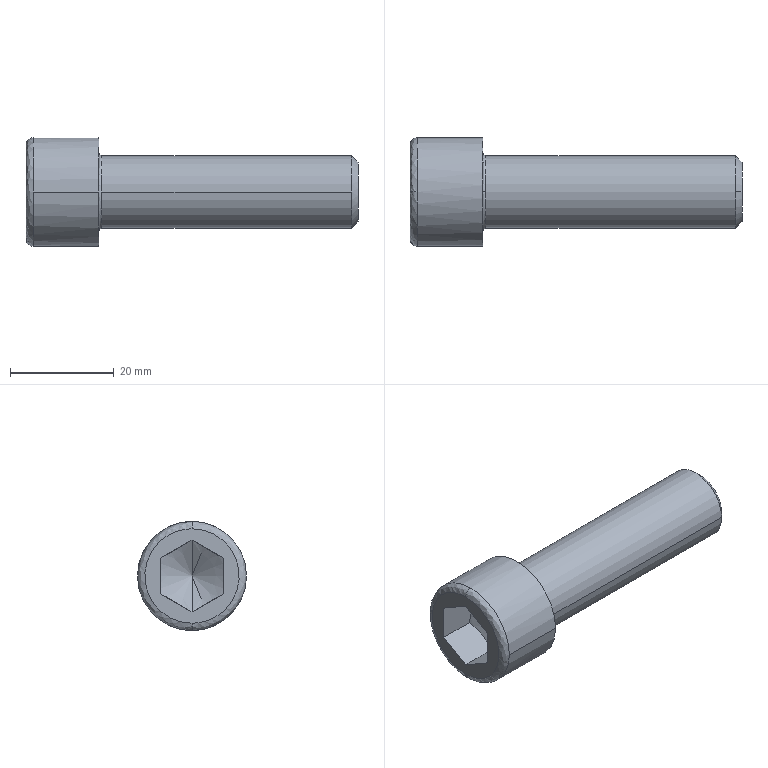Part | STEP file | Broached Socket Head Cap Screw - Metric M14x2 x 50 | 1 solid | 21 faces | box 64 x 21 x 21 mm | volume 11423 mm3 | plane 9 | spline 4 | cylinder 4 | cone 4 | commonest cylinder face diameters 14 x2 21 x2